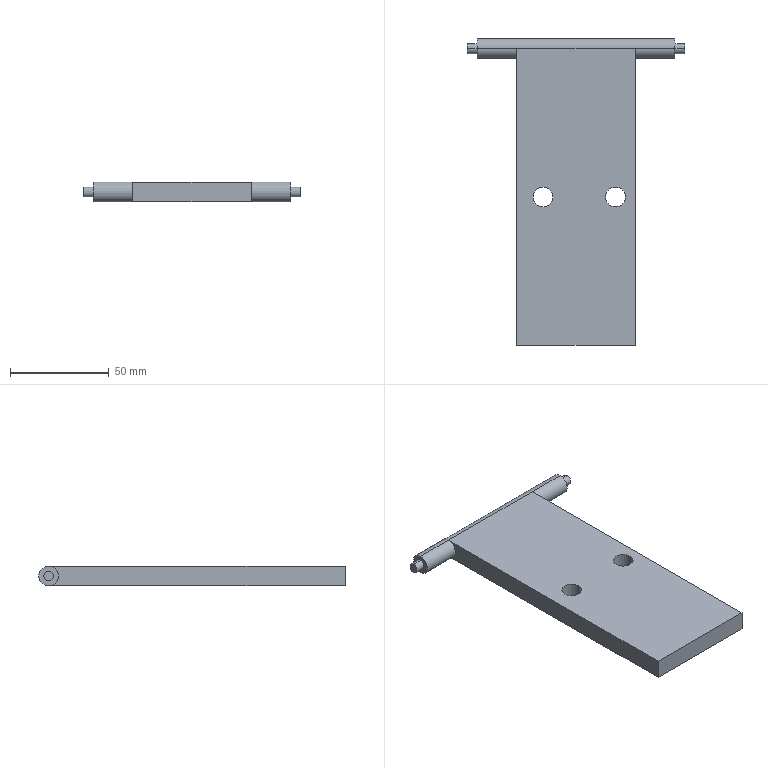Part | SolidWorks | features ICE 3, Extrusion 1 | 1 solid | 20 faces | box 110 x 155 x 10 mm | volume 94123 mm3 | cylinder 11 | plane 9 | commonest cylinder face diameters 10 x7 5 x4
STEP:
#1=CARTESIAN_POINT('',(-50.,75.,2.5));
#2=VERTEX_POINT('',#1);
#3=CARTESIAN_POINT('',(-50.,75.,7.5));
#4=VERTEX_POINT('',#3);
#5=CARTESIAN_POINT('',(-50.,75.,5.));
#6=DIRECTION('',(1.,0.,0.));
#7=DIRECTION('',(0.,0.,-1.));
#8=AXIS2_PLACEMENT_3D('',#5,#6,#7);
#9=CIRCLE('',#8,2.5);
#10=EDGE_CURVE('',#2,#4,#9,.T.);
#11=ORIENTED_EDGE('',*,*,#10,.F.);
#12=CARTESIAN_POINT('',(-55.,75.,2.5));
#13=VERTEX_POINT('',#12);
#14=CARTESIAN_POINT('',(55.,75.,2.5));
#15=DIRECTION('',(-1.,0.,0.));
#16=VECTOR('',#15,1000.);
#17=LINE('',#14,#16);
#18=EDGE_CURVE('',#2,#13,#17,.T.);
#19=ORIENTED_EDGE('',*,*,#18,.T.);
#20=CARTESIAN_POINT('',(-55.,75.,7.5));
#21=VERTEX_POINT('',#20);
#22=CARTESIAN_POINT('',(-55.,75.,5.));
#23=DIRECTION('',(-1.,0.,0.));
#24=DIRECTION('',(0.,0.,1.));
#25=AXIS2_PLACEMENT_3D('',#22,#23,#24);
#26=CIRCLE('',#25,2.5);
#27=EDGE_CURVE('',#21,#13,#26,.T.);
#28=ORIENTED_EDGE('',*,*,#27,.F.);
#29=CARTESIAN_POINT('',(55.,75.,7.5));
#30=DIRECTION('',(-1.,0.,0.));
#31=VECTOR('',#30,1000.);
#32=LINE('',#29,#31);
#33=EDGE_CURVE('',#4,#21,#32,.T.);
#34=ORIENTED_EDGE('',*,*,#33,.F.);
#35=EDGE_LOOP('',(#11,#19,#28,#34));
#36=FACE_OUTER_BOUND('',#35,.T.);
#37=CARTESIAN_POINT('',(55.,75.,5.));
#38=DIRECTION('',(-1.,0.,0.));
#39=DIRECTION('',(0.,0.,1.));
#40=AXIS2_PLACEMENT_3D('',#37,#38,#39);
#41=CYLINDRICAL_SURFACE('',#40,2.5);
#42=ADVANCED_FACE('',(#36),#41,.T.);
#43=CARTESIAN_POINT('',(55.,75.,7.5));
#44=VERTEX_POINT('',#43);
#45=CARTESIAN_POINT('',(55.,75.,2.5));
#46=VERTEX_POINT('',#45);
#47=CARTESIAN_POINT('',(55.,75.,5.));
#48=DIRECTION('',(-1.,0.,0.));
#49=DIRECTION('',(0.,0.,1.));
#50=AXIS2_PLACEMENT_3D('',#47,#48,#49);
#51=CIRCLE('',#50,2.5);
#52=EDGE_CURVE('',#44,#46,#51,.T.);
#53=ORIENTED_EDGE('',*,*,#52,.T.);
#54=CARTESIAN_POINT('',(50.,75.,2.5));
#55=VERTEX_POINT('',#54);
#56=CARTESIAN_POINT('',(55.,75.,2.5));
#57=DIRECTION('',(-1.,0.,0.));
#58=VECTOR('',#57,1000.);
#59=LINE('',#56,#58);
#60=EDGE_CURVE('',#46,#55,#59,.T.);
#61=ORIENTED_EDGE('',*,*,#60,.T.);
#62=CARTESIAN_POINT('',(50.,75.,7.5));
#63=VERTEX_POINT('',#62);
#64=CARTESIAN_POINT('',(50.,75.,5.));
#65=DIRECTION('',(1.,0.,0.));
#66=DIRECTION('',(0.,0.,-1.));
#67=AXIS2_PLACEMENT_3D('',#64,#65,#66);
#68=CIRCLE('',#67,2.5);
#69=EDGE_CURVE('',#55,#63,#68,.T.);
#70=ORIENTED_EDGE('',*,*,#69,.T.);
#71=CARTESIAN_POINT('',(55.,75.,7.5));
#72=DIRECTION('',(-1.,0.,0.));
#73=VECTOR('',#72,1000.);
#74=LINE('',#71,#73);
#75=EDGE_CURVE('',#44,#63,#74,.T.);
#76=ORIENTED_EDGE('',*,*,#75,.F.);
#77=EDGE_LOOP('',(#53,#61,#70,#76));
#78=FACE_OUTER_BOUND('',#77,.T.);
#79=CARTESIAN_POINT('',(55.,75.,5.));
#80=DIRECTION('',(-1.,0.,0.));
#81=DIRECTION('',(0.,0.,1.));
#82=AXIS2_PLACEMENT_3D('',#79,#80,#81);
#83=CYLINDRICAL_SURFACE('',#82,2.5);
#84=ADVANCED_FACE('',(#78),#83,.T.);
#85=CARTESIAN_POINT('',(-50.,75.,0.));
#86=VERTEX_POINT('',#85);
#87=CARTESIAN_POINT('',(-50.,75.,10.));
#88=VERTEX_POINT('',#87);
#89=CARTESIAN_POINT('',(-50.,75.,5.));
#90=DIRECTION('',(1.,0.,0.));
#91=DIRECTION('',(0.,0.,-1.));
#92=AXIS2_PLACEMENT_3D('',#89,#90,#91);
#93=CIRCLE('',#92,5.);
#94=EDGE_CURVE('',#86,#88,#93,.T.);
#95=ORIENTED_EDGE('',*,*,#94,.T.);
#96=CARTESIAN_POINT('',(-30.,75.,10.));
#97=VERTEX_POINT('',#96);
#98=CARTESIAN_POINT('',(-50.,75.,10.));
#99=DIRECTION('',(1.,0.,0.));
#100=VECTOR('',#99,1000.);
#101=LINE('',#98,#100);
#102=EDGE_CURVE('',#88,#97,#101,.T.);
#103=ORIENTED_EDGE('',*,*,#102,.T.);
#104=CARTESIAN_POINT('',(30.,75.,10.));
#105=VERTEX_POINT('',#104);
#106=CARTESIAN_POINT('',(30.,75.,10.));
#107=DIRECTION('',(-1.,0.,0.));
#108=VECTOR('',#107,1000.);
#109=LINE('',#106,#108);
#110=EDGE_CURVE('',#105,#97,#109,.T.);
#111=ORIENTED_EDGE('',*,*,#110,.F.);
#112=CARTESIAN_POINT('',(50.,75.,10.));
#113=VERTEX_POINT('',#112);
#114=CARTESIAN_POINT('',(-50.,75.,10.));
#115=DIRECTION('',(1.,0.,0.));
#116=VECTOR('',#115,1000.);
#117=LINE('',#114,#116);
#118=EDGE_CURVE('',#105,#113,#117,.T.);
#119=ORIENTED_EDGE('',*,*,#118,.T.);
#120=CARTESIAN_POINT('',(50.,75.,0.));
#121=VERTEX_POINT('',#120);
#122=CARTESIAN_POINT('',(50.,75.,5.));
#123=DIRECTION('',(1.,0.,0.));
#124=DIRECTION('',(0.,0.,-1.));
#125=AXIS2_PLACEMENT_3D('',#122,#123,#124);
#126=CIRCLE('',#125,5.);
#127=EDGE_CURVE('',#121,#113,#126,.T.);
#128=ORIENTED_EDGE('',*,*,#127,.F.);
#129=CARTESIAN_POINT('',(30.,75.,0.));
#130=VERTEX_POINT('',#129);
#131=CARTESIAN_POINT('',(-50.,75.,0.));
#132=DIRECTION('',(1.,0.,0.));
#133=VECTOR('',#132,1000.);
#134=LINE('',#131,#133);
#135=EDGE_CURVE('',#130,#121,#134,.T.);
#136=ORIENTED_EDGE('',*,*,#135,.F.);
#137=CARTESIAN_POINT('',(-30.,75.,0.));
#138=VERTEX_POINT('',#137);
#139=CARTESIAN_POINT('',(30.,75.,0.));
#140=DIRECTION('',(-1.,0.,0.));
#141=VECTOR('',#140,1000.);
#142=LINE('',#139,#141);
#143=EDGE_CURVE('',#130,#138,#142,.T.);
#144=ORIENTED_EDGE('',*,*,#143,.T.);
#145=CARTESIAN_POINT('',(-50.,75.,0.));
#146=DIRECTION('',(1.,0.,0.));
#147=VECTOR('',#146,1000.);
#148=LINE('',#145,#147);
#149=EDGE_CURVE('',#86,#138,#148,.T.);
#150=ORIENTED_EDGE('',*,*,#149,.F.);
#151=EDGE_LOOP('',(#95,#103,#111,#119,#128,#136,#144,#150));
#152=FACE_OUTER_BOUND('',#151,.T.);
#153=CARTESIAN_POINT('',(-50.,75.,5.));
#154=DIRECTION('',(1.,0.,0.));
#155=DIRECTION('',(0.,0.,-1.));
#156=AXIS2_PLACEMENT_3D('',#153,#154,#155);
#157=CYLINDRICAL_SURFACE('',#156,5.);
#158=ADVANCED_FACE('',(#152),#157,.T.);
#159=ORIENTED_EDGE('',*,*,#102,.F.);
#160=CARTESIAN_POINT('',(-50.,75.,5.));
#161=DIRECTION('',(1.,0.,0.));
#162=DIRECTION('',(0.,0.,-1.));
#163=AXIS2_PLACEMENT_3D('',#160,#161,#162);
#164=CIRCLE('',#163,5.);
#165=EDGE_CURVE('',#88,#86,#164,.T.);
#166=ORIENTED_EDGE('',*,*,#165,.T.);
#167=ORIENTED_EDGE('',*,*,#149,.T.);
#168=CARTESIAN_POINT('',(-30.,75.,5.));
#169=DIRECTION('',(1.,0.,0.));
#170=DIRECTION('',(0.,0.,-1.));
#171=AXIS2_PLACEMENT_3D('',#168,#169,#170);
#172=CIRCLE('',#171,5.);
#173=EDGE_CURVE('',#97,#138,#172,.T.);
#174=ORIENTED_EDGE('',*,*,#173,.F.);
#175=EDGE_LOOP('',(#159,#166,#167,#174));
#176=FACE_OUTER_BOUND('',#175,.T.);
#177=CARTESIAN_POINT('',(-50.,75.,5.));
#178=DIRECTION('',(1.,0.,0.));
#179=DIRECTION('',(0.,0.,-1.));
#180=AXIS2_PLACEMENT_3D('',#177,#178,#179);
#181=CYLINDRICAL_SURFACE('',#180,5.);
#182=ADVANCED_FACE('',(#176),#181,.T.);
#183=CARTESIAN_POINT('',(14.976,0.,0.));
#184=VERTEX_POINT('',#183);
#185=CARTESIAN_POINT('',(24.976,0.,0.));
#186=VERTEX_POINT('',#185);
#187=CARTESIAN_POINT('',(19.976,0.,0.));
#188=DIRECTION('',(0.,0.,1.));
#189=DIRECTION('',(1.,0.,0.));
#190=AXIS2_PLACEMENT_3D('',#187,#188,#189);
#191=CIRCLE('',#190,5.);
#192=EDGE_CURVE('',#184,#186,#191,.T.);
#193=ORIENTED_EDGE('',*,*,#192,.F.);
#194=CARTESIAN_POINT('',(14.976,0.,10.));
#195=VERTEX_POINT('',#194);
#196=CARTESIAN_POINT('',(14.976,0.,0.));
#197=DIRECTION('',(0.,0.,1.));
#198=VECTOR('',#197,1000.);
#199=LINE('',#196,#198);
#200=EDGE_CURVE('',#184,#195,#199,.T.);
#201=ORIENTED_EDGE('',*,*,#200,.T.);
#202=CARTESIAN_POINT('',(24.976,0.,10.));
#203=VERTEX_POINT('',#202);
#204=CARTESIAN_POINT('',(19.976,0.,10.));
#205=DIRECTION('',(0.,0.,1.));
#206=DIRECTION('',(1.,0.,0.));
#207=AXIS2_PLACEMENT_3D('',#204,#205,#206);
#208=CIRCLE('',#207,5.);
#209=EDGE_CURVE('',#195,#203,#208,.T.);
#210=ORIENTED_EDGE('',*,*,#209,.T.);
#211=CARTESIAN_POINT('',(24.976,0.,0.));
#212=DIRECTION('',(0.,0.,1.));
#213=VECTOR('',#212,1000.);
#214=LINE('',#211,#213);
#215=EDGE_CURVE('',#186,#203,#214,.T.);
#216=ORIENTED_EDGE('',*,*,#215,.F.);
#217=EDGE_LOOP('',(#193,#201,#210,#216));
#218=FACE_OUTER_BOUND('',#217,.T.);
#219=CARTESIAN_POINT('',(19.976,0.,0.));
#220=DIRECTION('',(0.,0.,1.));
#221=DIRECTION('',(1.,0.,0.));
#222=AXIS2_PLACEMENT_3D('',#219,#220,#221);
#223=CYLINDRICAL_SURFACE('',#222,5.);
#224=ADVANCED_FACE('',(#218),#223,.F.);
#225=CARTESIAN_POINT('',(-21.718,0.,0.));
#226=VERTEX_POINT('',#225);
#227=CARTESIAN_POINT('',(-11.718,0.,0.));
#228=VERTEX_POINT('',#227);
#229=CARTESIAN_POINT('',(-16.718,0.,0.));
#230=DIRECTION('',(0.,0.,1.));
#231=DIRECTION('',(1.,0.,0.));
#232=AXIS2_PLACEMENT_3D('',#229,#230,#231);
#233=CIRCLE('',#232,5.);
#234=EDGE_CURVE('',#226,#228,#233,.T.);
#235=ORIENTED_EDGE('',*,*,#234,.F.);
#236=CARTESIAN_POINT('',(-21.718,0.,10.));
#237=VERTEX_POINT('',#236);
#238=CARTESIAN_POINT('',(-21.718,0.,0.));
#239=DIRECTION('',(0.,0.,1.));
#240=VECTOR('',#239,1000.);
#241=LINE('',#238,#240);
#242=EDGE_CURVE('',#226,#237,#241,.T.);
#243=ORIENTED_EDGE('',*,*,#242,.T.);
#244=CARTESIAN_POINT('',(-11.718,0.,10.));
#245=VERTEX_POINT('',#244);
#246=CARTESIAN_POINT('',(-16.718,0.,10.));
#247=DIRECTION('',(0.,0.,1.));
#248=DIRECTION('',(1.,0.,0.));
#249=AXIS2_PLACEMENT_3D('',#246,#247,#248);
#250=CIRCLE('',#249,5.);
#251=EDGE_CURVE('',#237,#245,#250,.T.);
#252=ORIENTED_EDGE('',*,*,#251,.T.);
#253=CARTESIAN_POINT('',(-11.718,0.,0.));
#254=DIRECTION('',(0.,0.,1.));
#255=VECTOR('',#254,1000.);
#256=LINE('',#253,#255);
#257=EDGE_CURVE('',#228,#245,#256,.T.);
#258=ORIENTED_EDGE('',*,*,#257,.F.);
#259=EDGE_LOOP('',(#235,#243,#252,#258));
#260=FACE_OUTER_BOUND('',#259,.T.);
#261=CARTESIAN_POINT('',(-16.718,0.,0.));
#262=DIRECTION('',(0.,0.,1.));
#263=DIRECTION('',(1.,0.,0.));
#264=AXIS2_PLACEMENT_3D('',#261,#262,#263);
#265=CYLINDRICAL_SURFACE('',#264,5.);
#266=ADVANCED_FACE('',(#260),#265,.F.);
#267=CARTESIAN_POINT('',(-30.,-75.,10.));
#268=VERTEX_POINT('',#267);
#269=CARTESIAN_POINT('',(-30.,-75.,10.));
#270=DIRECTION('',(0.,-1.,0.));
#271=VECTOR('',#270,1000.);
#272=LINE('',#269,#271);
#273=EDGE_CURVE('',#97,#268,#272,.T.);
#274=ORIENTED_EDGE('',*,*,#273,.F.);
#275=ORIENTED_EDGE('',*,*,#173,.T.);
#276=CARTESIAN_POINT('',(-30.,-75.,0.));
#277=VERTEX_POINT('',#276);
#278=CARTESIAN_POINT('',(-30.,-75.,0.));
#279=DIRECTION('',(0.,-1.,0.));
#280=VECTOR('',#279,1000.);
#281=LINE('',#278,#280);
#282=EDGE_CURVE('',#138,#277,#281,.T.);
#283=ORIENTED_EDGE('',*,*,#282,.T.);
#284=CARTESIAN_POINT('',(-30.,-75.,10.));
#285=DIRECTION('',(0.,0.,-1.));
#286=VECTOR('',#285,1000.);
#287=LINE('',#284,#286);
#288=EDGE_CURVE('',#268,#277,#287,.T.);
#289=ORIENTED_EDGE('',*,*,#288,.F.);
#290=EDGE_LOOP('',(#274,#275,#283,#289));
#291=FACE_OUTER_BOUND('',#290,.T.);
#292=CARTESIAN_POINT('',(-30.,-75.,10.));
#293=DIRECTION('',(1.,0.,0.));
#294=DIRECTION('',(0.,0.,-1.));
#295=AXIS2_PLACEMENT_3D('',#292,#293,#294);
#296=PLANE('',#295);
#297=ADVANCED_FACE('',(#291),#296,.F.);
#298=CARTESIAN_POINT('',(30.,-75.,0.));
#299=VERTEX_POINT('',#298);
#300=CARTESIAN_POINT('',(30.,-75.,0.));
#301=DIRECTION('',(1.,0.,0.));
#302=VECTOR('',#301,1000.);
#303=LINE('',#300,#302);
#304=EDGE_CURVE('',#277,#299,#303,.T.);
#305=ORIENTED_EDGE('',*,*,#304,.T.);
#306=CARTESIAN_POINT('',(30.,-75.,10.));
#307=VERTEX_POINT('',#306);
#308=CARTESIAN_POINT('',(30.,-75.,10.));
#309=DIRECTION('',(0.,0.,-1.));
#310=VECTOR('',#309,1000.);
#311=LINE('',#308,#310);
#312=EDGE_CURVE('',#307,#299,#311,.T.);
#313=ORIENTED_EDGE('',*,*,#312,.F.);
#314=CARTESIAN_POINT('',(30.,-75.,10.));
#315=DIRECTION('',(1.,0.,0.));
#316=VECTOR('',#315,1000.);
#317=LINE('',#314,#316);
#318=EDGE_CURVE('',#268,#307,#317,.T.);
#319=ORIENTED_EDGE('',*,*,#318,.F.);
#320=ORIENTED_EDGE('',*,*,#288,.T.);
#321=EDGE_LOOP('',(#305,#313,#319,#320));
#322=FACE_OUTER_BOUND('',#321,.T.);
#323=CARTESIAN_POINT('',(30.,-75.,10.));
#324=DIRECTION('',(0.,1.,0.));
#325=DIRECTION('',(-1.,0.,0.));
#326=AXIS2_PLACEMENT_3D('',#323,#324,#325);
#327=PLANE('',#326);
#328=ADVANCED_FACE('',(#322),#327,.F.);
#329=CARTESIAN_POINT('',(30.,-75.,0.));
#330=DIRECTION('',(0.,1.,0.));
#331=VECTOR('',#330,1000.);
#332=LINE('',#329,#331);
#333=EDGE_CURVE('',#299,#130,#332,.T.);
#334=ORIENTED_EDGE('',*,*,#333,.T.);
#335=CARTESIAN_POINT('',(30.,75.,5.));
#336=DIRECTION('',(-1.,0.,0.));
#337=DIRECTION('',(0.,0.,1.));
#338=AXIS2_PLACEMENT_3D('',#335,#336,#337);
#339=CIRCLE('',#338,5.);
#340=EDGE_CURVE('',#130,#105,#339,.T.);
#341=ORIENTED_EDGE('',*,*,#340,.T.);
#342=CARTESIAN_POINT('',(30.,-75.,10.));
#343=DIRECTION('',(0.,1.,0.));
#344=VECTOR('',#343,1000.);
#345=LINE('',#342,#344);
#346=EDGE_CURVE('',#307,#105,#345,.T.);
#347=ORIENTED_EDGE('',*,*,#346,.F.);
#348=ORIENTED_EDGE('',*,*,#312,.T.);
#349=EDGE_LOOP('',(#334,#341,#347,#348));
#350=FACE_OUTER_BOUND('',#349,.T.);
#351=CARTESIAN_POINT('',(30.,-75.,10.));
#352=DIRECTION('',(-1.,0.,0.));
#353=DIRECTION('',(0.,0.,1.));
#354=AXIS2_PLACEMENT_3D('',#351,#352,#353);
#355=PLANE('',#354);
#356=ADVANCED_FACE('',(#350),#355,.F.);
#357=CARTESIAN_POINT('',(19.976,0.,10.));
#358=DIRECTION('',(0.,0.,1.));
#359=DIRECTION('',(1.,0.,0.));
#360=AXIS2_PLACEMENT_3D('',#357,#358,#359);
#361=CIRCLE('',#360,5.);
#362=EDGE_CURVE('',#203,#195,#361,.T.);
#363=ORIENTED_EDGE('',*,*,#362,.F.);
#364=ORIENTED_EDGE('',*,*,#209,.F.);
#365=EDGE_LOOP('',(#363,#364));
#366=FACE_BOUND('',#365,.T.);
#367=CARTESIAN_POINT('',(-16.718,0.,10.));
#368=DIRECTION('',(0.,0.,1.));
#369=DIRECTION('',(1.,0.,0.));
#370=AXIS2_PLACEMENT_3D('',#367,#368,#369);
#371=CIRCLE('',#370,5.);
#372=EDGE_CURVE('',#245,#237,#371,.T.);
#373=ORIENTED_EDGE('',*,*,#372,.F.);
#374=ORIENTED_EDGE('',*,*,#251,.F.);
#375=EDGE_LOOP('',(#373,#374));
#376=FACE_BOUND('',#375,.T.);
#377=ORIENTED_EDGE('',*,*,#273,.T.);
#378=ORIENTED_EDGE('',*,*,#318,.T.);
#379=ORIENTED_EDGE('',*,*,#346,.T.);
#380=ORIENTED_EDGE('',*,*,#110,.T.);
#381=EDGE_LOOP('',(#377,#378,#379,#380));
#382=FACE_OUTER_BOUND('',#381,.T.);
#383=CARTESIAN_POINT('',(-30.,75.,10.));
#384=DIRECTION('',(0.,0.,1.));
#385=DIRECTION('',(1.,0.,0.));
#386=AXIS2_PLACEMENT_3D('',#383,#384,#385);
#387=PLANE('',#386);
#388=ADVANCED_FACE('',(#366,#376,#382),#387,.T.);
#389=CARTESIAN_POINT('',(19.976,0.,0.));
#390=DIRECTION('',(0.,0.,1.));
#391=DIRECTION('',(1.,0.,0.));
#392=AXIS2_PLACEMENT_3D('',#389,#390,#391);
#393=CIRCLE('',#392,5.);
#394=EDGE_CURVE('',#186,#184,#393,.T.);
#395=ORIENTED_EDGE('',*,*,#394,.T.);
#396=ORIENTED_EDGE('',*,*,#192,.T.);
#397=EDGE_LOOP('',(#395,#396));
#398=FACE_BOUND('',#397,.T.);
#399=CARTESIAN_POINT('',(-16.718,0.,0.));
#400=DIRECTION('',(0.,0.,1.));
#401=DIRECTION('',(1.,0.,0.));
#402=AXIS2_PLACEMENT_3D('',#399,#400,#401);
#403=CIRCLE('',#402,5.);
#404=EDGE_CURVE('',#228,#226,#403,.T.);
#405=ORIENTED_EDGE('',*,*,#404,.T.);
#406=ORIENTED_EDGE('',*,*,#234,.T.);
#407=EDGE_LOOP('',(#405,#406));
#408=FACE_BOUND('',#407,.T.);
#409=ORIENTED_EDGE('',*,*,#282,.F.);
#410=ORIENTED_EDGE('',*,*,#143,.F.);
#411=ORIENTED_EDGE('',*,*,#333,.F.);
#412=ORIENTED_EDGE('',*,*,#304,.F.);
#413=EDGE_LOOP('',(#409,#410,#411,#412));
#414=FACE_OUTER_BOUND('',#413,.T.);
#415=CARTESIAN_POINT('',(-30.,75.,0.));
#416=DIRECTION('',(0.,0.,1.));
#417=DIRECTION('',(1.,0.,0.));
#418=AXIS2_PLACEMENT_3D('',#415,#416,#417);
#419=PLANE('',#418);
#420=ADVANCED_FACE('',(#398,#408,#414),#419,.F.);
#421=ORIENTED_EDGE('',*,*,#242,.F.);
#422=ORIENTED_EDGE('',*,*,#404,.F.);
#423=ORIENTED_EDGE('',*,*,#257,.T.);
#424=ORIENTED_EDGE('',*,*,#372,.T.);
#425=EDGE_LOOP('',(#421,#422,#423,#424));
#426=FACE_OUTER_BOUND('',#425,.T.);
#427=CARTESIAN_POINT('',(-16.718,0.,0.));
#428=DIRECTION('',(0.,0.,1.));
#429=DIRECTION('',(1.,0.,0.));
#430=AXIS2_PLACEMENT_3D('',#427,#428,#429);
#431=CYLINDRICAL_SURFACE('',#430,5.);
#432=ADVANCED_FACE('',(#426),#431,.F.);
#433=ORIENTED_EDGE('',*,*,#200,.F.);
#434=ORIENTED_EDGE('',*,*,#394,.F.);
#435=ORIENTED_EDGE('',*,*,#215,.T.);
#436=ORIENTED_EDGE('',*,*,#362,.T.);
#437=EDGE_LOOP('',(#433,#434,#435,#436));
#438=FACE_OUTER_BOUND('',#437,.T.);
#439=CARTESIAN_POINT('',(19.976,0.,0.));
#440=DIRECTION('',(0.,0.,1.));
#441=DIRECTION('',(1.,0.,0.));
#442=AXIS2_PLACEMENT_3D('',#439,#440,#441);
#443=CYLINDRICAL_SURFACE('',#442,5.);
#444=ADVANCED_FACE('',(#438),#443,.F.);
#445=ORIENTED_EDGE('',*,*,#118,.F.);
#446=ORIENTED_EDGE('',*,*,#340,.F.);
#447=ORIENTED_EDGE('',*,*,#135,.T.);
#448=CARTESIAN_POINT('',(50.,75.,5.));
#449=DIRECTION('',(1.,0.,0.));
#450=DIRECTION('',(0.,0.,-1.));
#451=AXIS2_PLACEMENT_3D('',#448,#449,#450);
#452=CIRCLE('',#451,5.);
#453=EDGE_CURVE('',#113,#121,#452,.T.);
#454=ORIENTED_EDGE('',*,*,#453,.F.);
#455=EDGE_LOOP('',(#445,#446,#447,#454));
#456=FACE_OUTER_BOUND('',#455,.T.);
#457=CARTESIAN_POINT('',(-50.,75.,5.));
#458=DIRECTION('',(1.,0.,0.));
#459=DIRECTION('',(0.,0.,-1.));
#460=AXIS2_PLACEMENT_3D('',#457,#458,#459);
#461=CYLINDRICAL_SURFACE('',#460,5.);
#462=ADVANCED_FACE('',(#456),#461,.T.);
#463=CARTESIAN_POINT('',(-50.,75.,5.));
#464=DIRECTION('',(1.,0.,0.));
#465=DIRECTION('',(0.,0.,-1.));
#466=AXIS2_PLACEMENT_3D('',#463,#464,#465);
#467=CIRCLE('',#466,2.5);
#468=EDGE_CURVE('',#4,#2,#467,.T.);
#469=ORIENTED_EDGE('',*,*,#468,.T.);
#470=ORIENTED_EDGE('',*,*,#10,.T.);
#471=EDGE_LOOP('',(#469,#470));
#472=FACE_BOUND('',#471,.T.);
#473=ORIENTED_EDGE('',*,*,#94,.F.);
#474=ORIENTED_EDGE('',*,*,#165,.F.);
#475=EDGE_LOOP('',(#473,#474));
#476=FACE_OUTER_BOUND('',#475,.T.);
#477=CARTESIAN_POINT('',(-50.,75.,5.));
#478=DIRECTION('',(1.,0.,0.));
#479=DIRECTION('',(0.,0.,-1.));
#480=AXIS2_PLACEMENT_3D('',#477,#478,#479);
#481=PLANE('',#480);
#482=ADVANCED_FACE('',(#472,#476),#481,.F.);
#483=CARTESIAN_POINT('',(50.,75.,5.));
#484=DIRECTION('',(1.,0.,0.));
#485=DIRECTION('',(0.,0.,-1.));
#486=AXIS2_PLACEMENT_3D('',#483,#484,#485);
#487=CIRCLE('',#486,2.5);
#488=EDGE_CURVE('',#63,#55,#487,.T.);
#489=ORIENTED_EDGE('',*,*,#488,.F.);
#490=ORIENTED_EDGE('',*,*,#69,.F.);
#491=EDGE_LOOP('',(#489,#490));
#492=FACE_BOUND('',#491,.T.);
#493=ORIENTED_EDGE('',*,*,#127,.T.);
#494=ORIENTED_EDGE('',*,*,#453,.T.);
#495=EDGE_LOOP('',(#493,#494));
#496=FACE_OUTER_BOUND('',#495,.T.);
#497=CARTESIAN_POINT('',(50.,75.,5.));
#498=DIRECTION('',(1.,0.,0.));
#499=DIRECTION('',(0.,0.,-1.));
#500=AXIS2_PLACEMENT_3D('',#497,#498,#499);
#501=PLANE('',#500);
#502=ADVANCED_FACE('',(#492,#496),#501,.T.);
#503=ORIENTED_EDGE('',*,*,#52,.F.);
#504=CARTESIAN_POINT('',(55.,75.,5.));
#505=DIRECTION('',(-1.,0.,0.));
#506=DIRECTION('',(0.,0.,1.));
#507=AXIS2_PLACEMENT_3D('',#504,#505,#506);
#508=CIRCLE('',#507,2.5);
#509=EDGE_CURVE('',#46,#44,#508,.T.);
#510=ORIENTED_EDGE('',*,*,#509,.F.);
#511=EDGE_LOOP('',(#503,#510));
#512=FACE_OUTER_BOUND('',#511,.T.);
#513=CARTESIAN_POINT('',(55.,75.,5.));
#514=DIRECTION('',(-1.,0.,0.));
#515=DIRECTION('',(0.,0.,1.));
#516=AXIS2_PLACEMENT_3D('',#513,#514,#515);
#517=PLANE('',#516);
#518=ADVANCED_FACE('',(#512),#517,.F.);
#519=ORIENTED_EDGE('',*,*,#60,.F.);
#520=ORIENTED_EDGE('',*,*,#509,.T.);
#521=ORIENTED_EDGE('',*,*,#75,.T.);
#522=ORIENTED_EDGE('',*,*,#488,.T.);
#523=EDGE_LOOP('',(#519,#520,#521,#522));
#524=FACE_OUTER_BOUND('',#523,.T.);
#525=CARTESIAN_POINT('',(55.,75.,5.));
#526=DIRECTION('',(-1.,0.,0.));
#527=DIRECTION('',(0.,0.,1.));
#528=AXIS2_PLACEMENT_3D('',#525,#526,#527);
#529=CYLINDRICAL_SURFACE('',#528,2.5);
#530=ADVANCED_FACE('',(#524),#529,.T.);
#531=ORIENTED_EDGE('',*,*,#18,.F.);
#532=ORIENTED_EDGE('',*,*,#468,.F.);
#533=ORIENTED_EDGE('',*,*,#33,.T.);
#534=CARTESIAN_POINT('',(-55.,75.,5.));
#535=DIRECTION('',(-1.,0.,0.));
#536=DIRECTION('',(0.,0.,1.));
#537=AXIS2_PLACEMENT_3D('',#534,#535,#536);
#538=CIRCLE('',#537,2.5);
#539=EDGE_CURVE('',#13,#21,#538,.T.);
#540=ORIENTED_EDGE('',*,*,#539,.F.);
#541=EDGE_LOOP('',(#531,#532,#533,#540));
#542=FACE_OUTER_BOUND('',#541,.T.);
#543=CARTESIAN_POINT('',(55.,75.,5.));
#544=DIRECTION('',(-1.,0.,0.));
#545=DIRECTION('',(0.,0.,1.));
#546=AXIS2_PLACEMENT_3D('',#543,#544,#545);
#547=CYLINDRICAL_SURFACE('',#546,2.5);
#548=ADVANCED_FACE('',(#542),#547,.T.);
#549=ORIENTED_EDGE('',*,*,#27,.T.);
#550=ORIENTED_EDGE('',*,*,#539,.T.);
#551=EDGE_LOOP('',(#549,#550));
#552=FACE_OUTER_BOUND('',#551,.T.);
#553=CARTESIAN_POINT('',(-55.,75.,5.));
#554=DIRECTION('',(-1.,0.,0.));
#555=DIRECTION('',(0.,0.,1.));
#556=AXIS2_PLACEMENT_3D('',#553,#554,#555);
#557=PLANE('',#556);
#558=ADVANCED_FACE('',(#552),#557,.T.);
#559=CLOSED_SHELL('',(#42,#84,#158,#182,#224,#266,#297,#328,#356,#388,#420,#432,#444,#462,#482,#502,#518,#530,#548,#558));
#560=MANIFOLD_SOLID_BREP('',#559);
#561=CARTESIAN_POINT('',(0.,0.,0.));
#562=DIRECTION('',(0.,0.,1.));
#563=DIRECTION('',(1.,0.,0.));
#564=AXIS2_PLACEMENT_3D('',#561,#562,#563);
#565=(LENGTH_UNIT()NAMED_UNIT(*)SI_UNIT(.MILLI.,.METRE.));
#566=UNCERTAINTY_MEASURE_WITH_UNIT(LENGTH_MEASURE(0.00001),#565,'','');
#567=(NAMED_UNIT(*)PLANE_ANGLE_UNIT()SI_UNIT($,.RADIAN.));
#568=(NAMED_UNIT(*)SI_UNIT($,.STERADIAN.)SOLID_ANGLE_UNIT());
#569=(GEOMETRIC_REPRESENTATION_CONTEXT(3)GLOBAL_UNCERTAINTY_ASSIGNED_CONTEXT((#566))GLOBAL_UNIT_ASSIGNED_CONTEXT((#565,#567,#568))REPRESENTATION_CONTEXT('',''));
#570=ADVANCED_BREP_SHAPE_REPRESENTATION('',(#560,#564),#569);